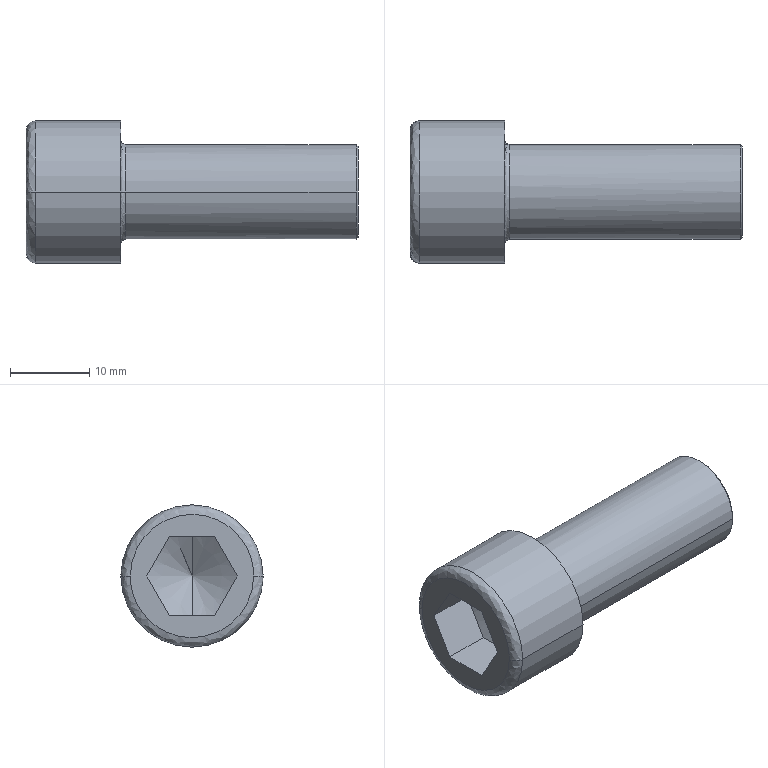Part | SolidWorks | features BaseBody 1 | 1 solid | 27 faces | box 42 x 18 x 18 mm | volume 5810 mm3 | plane 15 | spline 4 | cylinder 4 | cone 4 | commonest cylinder face diameters 12 x2 18 x2
STEP:
#1=CARTESIAN_POINT('',(0.6,6.,0.));
#2=VERTEX_POINT('',#1);
#3=CARTESIAN_POINT('',(0.6,-6.,0.));
#4=VERTEX_POINT('',#3);
#5=CARTESIAN_POINT('',(0.6,0.,0.));
#6=DIRECTION('',(1.,0.,0.));
#7=DIRECTION('',(0.,-1.,0.));
#8=AXIS2_PLACEMENT_3D('',#5,#6,#7);
#9=CIRCLE('',#8,6.);
#10=EDGE_CURVE('',#2,#4,#9,.T.);
#11=ORIENTED_EDGE('',*,*,#10,.F.);
#12=CARTESIAN_POINT('',(0.,6.6,0.));
#13=VERTEX_POINT('',#12);
#14=CARTESIAN_POINT('',(0.6,6.6,0.));
#15=DIRECTION('',(0.,0.,-1.));
#16=DIRECTION('',(0.,1.,0.));
#17=AXIS2_PLACEMENT_3D('',#14,#15,#16);
#18=CIRCLE('',#17,0.6);
#19=EDGE_CURVE('',#2,#13,#18,.T.);
#20=ORIENTED_EDGE('',*,*,#19,.T.);
#21=CARTESIAN_POINT('',(0.,-6.6,0.));
#22=VERTEX_POINT('',#21);
#23=CARTESIAN_POINT('',(0.,-6.6,0.));
#24=CARTESIAN_POINT('',(0.,-6.6,0.2019));
#25=CARTESIAN_POINT('',(0.,-6.586,0.5035));
#26=CARTESIAN_POINT('',(0.,-6.546,0.853));
#27=CARTESIAN_POINT('',(0.,-6.52,1.027));
#28=CARTESIAN_POINT('',(0.,-6.507,1.102));
#29=CARTESIAN_POINT('',(0.,-6.499,1.151));
#30=CARTESIAN_POINT('',(0.,-6.495,1.175));
#31=CARTESIAN_POINT('',(0.,-6.451,1.412));
#32=CARTESIAN_POINT('',(0.,-6.377,1.723));
#33=CARTESIAN_POINT('',(0.,-6.266,2.079));
#34=CARTESIAN_POINT('',(0.,-6.203,2.255));
#35=CARTESIAN_POINT('',(0.,-6.175,2.33));
#36=CARTESIAN_POINT('',(0.,-6.156,2.38));
#37=CARTESIAN_POINT('',(0.,-6.147,2.403));
#38=CARTESIAN_POINT('',(0.,-6.054,2.637));
#39=CARTESIAN_POINT('',(0.,-5.916,2.94));
#40=CARTESIAN_POINT('',(0.,-5.729,3.281));
#41=CARTESIAN_POINT('',(0.,-5.643,3.423));
#42=CARTESIAN_POINT('',(0.,-5.585,3.518));
#43=CARTESIAN_POINT('',(0.,-5.555,3.564));
#44=CARTESIAN_POINT('',(0.,-5.275,3.993));
#45=CARTESIAN_POINT('',(0.,-4.989,4.344));
#46=CARTESIAN_POINT('',(0.,-4.506,4.828));
#47=CARTESIAN_POINT('',(0.,-4.253,5.056));
#48=CARTESIAN_POINT('',(0.,-3.984,5.264));
#49=CARTESIAN_POINT('',(0.,-3.8,5.397));
#50=CARTESIAN_POINT('',(0.,-3.705,5.463));
#51=CARTESIAN_POINT('',(0.,-3.425,5.646));
#52=CARTESIAN_POINT('',(0.,-3.137,5.814));
#53=CARTESIAN_POINT('',(0.,-2.788,5.984));
#54=CARTESIAN_POINT('',(0.,-2.635,6.051));
#55=CARTESIAN_POINT('',(0.,-2.533,6.095));
#56=CARTESIAN_POINT('',(0.,-2.479,6.117));
#57=CARTESIAN_POINT('',(0.,-2.23,6.215));
#58=CARTESIAN_POINT('',(0.,-1.927,6.319));
#59=CARTESIAN_POINT('',(0.,-1.567,6.413));
#60=CARTESIAN_POINT('',(0.,-1.384,6.454));
#61=CARTESIAN_POINT('',(0.,-1.306,6.47));
#62=CARTESIAN_POINT('',(0.,-1.253,6.48));
#63=CARTESIAN_POINT('',(0.,-1.226,6.485));
#64=CARTESIAN_POINT('',(0.,-0.8037,6.563));
#65=CARTESIAN_POINT('',(0.,-0.404,6.6));
#66=CARTESIAN_POINT('',(0.,0.202,6.6));
#67=CARTESIAN_POINT('',(0.,0.5037,6.586));
#68=CARTESIAN_POINT('',(0.,0.8531,6.546));
#69=CARTESIAN_POINT('',(0.,1.027,6.52));
#70=CARTESIAN_POINT('',(0.,1.102,6.507));
#71=CARTESIAN_POINT('',(0.,1.151,6.499));
#72=CARTESIAN_POINT('',(0.,1.175,6.495));
#73=CARTESIAN_POINT('',(0.,1.412,6.451));
#74=CARTESIAN_POINT('',(0.,1.723,6.377));
#75=CARTESIAN_POINT('',(0.,2.079,6.266));
#76=CARTESIAN_POINT('',(0.,2.255,6.203));
#77=CARTESIAN_POINT('',(0.,2.33,6.175));
#78=CARTESIAN_POINT('',(0.,2.38,6.156));
#79=CARTESIAN_POINT('',(0.,2.403,6.147));
#80=CARTESIAN_POINT('',(0.,2.637,6.054));
#81=CARTESIAN_POINT('',(0.,2.94,5.916));
#82=CARTESIAN_POINT('',(0.,3.281,5.729));
#83=CARTESIAN_POINT('',(0.,3.423,5.643));
#84=CARTESIAN_POINT('',(0.,3.518,5.585));
#85=CARTESIAN_POINT('',(0.,3.564,5.555));
#86=CARTESIAN_POINT('',(0.,3.993,5.275));
#87=CARTESIAN_POINT('',(0.,4.344,4.989));
#88=CARTESIAN_POINT('',(0.,4.828,4.506));
#89=CARTESIAN_POINT('',(0.,5.056,4.253));
#90=CARTESIAN_POINT('',(0.,5.264,3.984));
#91=CARTESIAN_POINT('',(0.,5.397,3.8));
#92=CARTESIAN_POINT('',(0.,5.463,3.705));
#93=CARTESIAN_POINT('',(0.,5.646,3.425));
#94=CARTESIAN_POINT('',(0.,5.814,3.137));
#95=CARTESIAN_POINT('',(0.,5.984,2.788));
#96=CARTESIAN_POINT('',(0.,6.051,2.635));
#97=CARTESIAN_POINT('',(0.,6.095,2.533));
#98=CARTESIAN_POINT('',(0.,6.117,2.479));
#99=CARTESIAN_POINT('',(0.,6.215,2.23));
#100=CARTESIAN_POINT('',(0.,6.319,1.927));
#101=CARTESIAN_POINT('',(0.,6.413,1.567));
#102=CARTESIAN_POINT('',(0.,6.454,1.384));
#103=CARTESIAN_POINT('',(0.,6.47,1.306));
#104=CARTESIAN_POINT('',(0.,6.48,1.253));
#105=CARTESIAN_POINT('',(0.,6.485,1.226));
#106=CARTESIAN_POINT('',(0.,6.563,0.8038));
#107=CARTESIAN_POINT('',(0.,6.6,0.4035));
#108=CARTESIAN_POINT('',(0.,6.6,0.));
#109=B_SPLINE_CURVE_WITH_KNOTS('',3,(#23,#24,#25,#26,#27,#28,#29,#30,#31,#32,#33,#34,#35,#36,#37,#38,#39,#40,#41,#42,#43,#44,#45,#46,#47,#48,#49,#50,#51,#52,#53,#54,#55,#56,#57,#58,#59,#60,#61,#62,#63,#64,#65,#66,#67,#68,#69,#70,#71,#72,#73,#74,#75,#76,#77,#78,#79,#80,#81,#82,#83,#84,#85,#86,#87,#88,#89,#90,#91,#92,#93,#94,#95,#96,#97,#98,#99,#100,#101,#102,#103,#104,#105,#106,#107,#108),.UNSPECIFIED.,.F.,.F.,(4,1,1,1,2,2,1,1,1,2,2,1,1,2,2,2,1,2,2,1,1,2,2,1,1,1,2,2,2,1,1,1,2,2,1,1,1,2,2,1,1,2,2,2,1,2,2,1,1,2,2,1,1,1,2,2,4),(0.,0.03125,0.04688,0.05469,0.05859,0.0625,0.09375,0.1094,0.1172,0.1211,0.125,0.1563,0.1719,0.1797,0.1875,0.25,0.2813,0.2969,0.3125,0.3438,0.3594,0.3672,0.375,0.4063,0.4219,0.4297,0.4336,0.4375,0.5,0.5313,0.5469,0.5547,0.5586,0.5625,0.5938,0.6094,0.6172,0.6211,0.625,0.6563,0.6719,0.6797,0.6875,0.75,0.7813,0.7969,0.8125,0.8438,0.8594,0.8672,0.875,0.9063,0.9219,0.9297,0.9336,0.9375,1.),.UNSPECIFIED.);
#110=EDGE_CURVE('',#22,#13,#109,.T.);
#111=ORIENTED_EDGE('',*,*,#110,.F.);
#112=CARTESIAN_POINT('',(0.6,-6.6,0.));
#113=DIRECTION('',(0.,0.,1.));
#114=DIRECTION('',(0.,-1.,0.));
#115=AXIS2_PLACEMENT_3D('',#112,#113,#114);
#116=CIRCLE('',#115,0.6);
#117=EDGE_CURVE('',#4,#22,#116,.T.);
#118=ORIENTED_EDGE('',*,*,#117,.F.);
#119=EDGE_LOOP('',(#11,#20,#111,#118));
#120=FACE_OUTER_BOUND('',#119,.T.);
#121=CARTESIAN_POINT('',(0.6,-6.,0.));
#122=CARTESIAN_POINT('',(0.6,-6.,12.));
#123=CARTESIAN_POINT('',(0.6,6.,12.));
#124=CARTESIAN_POINT('',(0.6,6.,0.));
#125=CARTESIAN_POINT('',(0.2485,-6.,0.));
#126=CARTESIAN_POINT('',(0.2485,-6.,12.));
#127=CARTESIAN_POINT('',(0.2485,6.,12.));
#128=CARTESIAN_POINT('',(0.2485,6.,0.));
#129=CARTESIAN_POINT('',(0.,-6.249,0.));
#130=CARTESIAN_POINT('',(0.,-6.249,12.497));
#131=CARTESIAN_POINT('',(0.,6.249,12.497));
#132=CARTESIAN_POINT('',(0.,6.249,0.));
#133=CARTESIAN_POINT('',(0.,-6.6,0.));
#134=CARTESIAN_POINT('',(0.,-6.6,13.2));
#135=CARTESIAN_POINT('',(0.,6.6,13.2));
#136=CARTESIAN_POINT('',(0.,6.6,0.));
#137=(BOUNDED_SURFACE()B_SPLINE_SURFACE(3,3,((#121,#122,#123,#124),(#125,#126,#127,#128),(#129,#130,#131,#132),(#133,#134,#135,#136)),.UNSPECIFIED.,.F.,.F.,.T.)B_SPLINE_SURFACE_WITH_KNOTS((4,4),(4,4),(0.,1.),(0.,1.),.UNSPECIFIED.)GEOMETRIC_REPRESENTATION_ITEM()RATIONAL_B_SPLINE_SURFACE(((1.,0.3333,0.3333,1.),(0.8047,0.2682,0.2682,0.8047),(0.8047,0.2682,0.2682,0.8047),(1.,0.3333,0.3333,1.)))REPRESENTATION_ITEM('')SURFACE());
#138=ADVANCED_FACE('',(#120),#137,.F.);
#139=CARTESIAN_POINT('',(-10.8,-9.,0.));
#140=VERTEX_POINT('',#139);
#141=CARTESIAN_POINT('',(-10.8,9.,0.));
#142=VERTEX_POINT('',#141);
#143=CARTESIAN_POINT('',(-10.8,0.,0.));
#144=DIRECTION('',(1.,0.,0.));
#145=DIRECTION('',(0.,-1.,0.));
#146=AXIS2_PLACEMENT_3D('',#143,#144,#145);
#147=CIRCLE('',#146,9.);
#148=EDGE_CURVE('',#140,#142,#147,.T.);
#149=ORIENTED_EDGE('',*,*,#148,.F.);
#150=CARTESIAN_POINT('',(-12.,-7.8,0.));
#151=VERTEX_POINT('',#150);
#152=CARTESIAN_POINT('',(-10.8,-7.8,0.));
#153=DIRECTION('',(0.,0.,-1.));
#154=DIRECTION('',(0.,-1.,0.));
#155=AXIS2_PLACEMENT_3D('',#152,#153,#154);
#156=CIRCLE('',#155,1.2);
#157=EDGE_CURVE('',#140,#151,#156,.T.);
#158=ORIENTED_EDGE('',*,*,#157,.T.);
#159=CARTESIAN_POINT('',(-12.,7.8,0.));
#160=VERTEX_POINT('',#159);
#161=CARTESIAN_POINT('',(-12.,-7.8,0.));
#162=CARTESIAN_POINT('',(-12.,-7.8,-15.6));
#163=CARTESIAN_POINT('',(-12.,7.8,-15.6));
#164=CARTESIAN_POINT('',(-12.,7.8,0.));
#165=(BOUNDED_CURVE()B_SPLINE_CURVE(3,(#161,#162,#163,#164),.UNSPECIFIED.,.F.,.T.)B_SPLINE_CURVE_WITH_KNOTS((4,4),(0.,1.),.UNSPECIFIED.)CURVE()GEOMETRIC_REPRESENTATION_ITEM()RATIONAL_B_SPLINE_CURVE((1.,0.3333,0.3333,1.))REPRESENTATION_ITEM(''));
#166=EDGE_CURVE('',#151,#160,#165,.T.);
#167=ORIENTED_EDGE('',*,*,#166,.T.);
#168=CARTESIAN_POINT('',(-10.8,7.8,0.));
#169=DIRECTION('',(0.,0.,1.));
#170=DIRECTION('',(0.,1.,0.));
#171=AXIS2_PLACEMENT_3D('',#168,#169,#170);
#172=CIRCLE('',#171,1.2);
#173=EDGE_CURVE('',#142,#160,#172,.T.);
#174=ORIENTED_EDGE('',*,*,#173,.F.);
#175=EDGE_LOOP('',(#149,#158,#167,#174));
#176=FACE_OUTER_BOUND('',#175,.T.);
#177=CARTESIAN_POINT('',(-10.8,-9.,0.));
#178=CARTESIAN_POINT('',(-10.8,-9.,-18.));
#179=CARTESIAN_POINT('',(-10.8,9.,-18.));
#180=CARTESIAN_POINT('',(-10.8,9.,0.));
#181=CARTESIAN_POINT('',(-11.503,-9.,0.));
#182=CARTESIAN_POINT('',(-11.503,-9.,-18.));
#183=CARTESIAN_POINT('',(-11.503,9.,-18.));
#184=CARTESIAN_POINT('',(-11.503,9.,0.));
#185=CARTESIAN_POINT('',(-12.,-8.503,0.));
#186=CARTESIAN_POINT('',(-12.,-8.503,-17.006));
#187=CARTESIAN_POINT('',(-12.,8.503,-17.006));
#188=CARTESIAN_POINT('',(-12.,8.503,0.));
#189=CARTESIAN_POINT('',(-12.,-7.8,0.));
#190=CARTESIAN_POINT('',(-12.,-7.8,-15.6));
#191=CARTESIAN_POINT('',(-12.,7.8,-15.6));
#192=CARTESIAN_POINT('',(-12.,7.8,0.));
#193=(BOUNDED_SURFACE()B_SPLINE_SURFACE(3,3,((#177,#178,#179,#180),(#181,#182,#183,#184),(#185,#186,#187,#188),(#189,#190,#191,#192)),.UNSPECIFIED.,.F.,.F.,.F.)B_SPLINE_SURFACE_WITH_KNOTS((4,4),(4,4),(0.,1.),(0.,1.),.UNSPECIFIED.)GEOMETRIC_REPRESENTATION_ITEM()RATIONAL_B_SPLINE_SURFACE(((1.,0.3333,0.3333,1.),(0.8047,0.2682,0.2682,0.8047),(0.8047,0.2682,0.2682,0.8047),(1.,0.3333,0.3333,1.)))REPRESENTATION_ITEM('')SURFACE());
#194=ADVANCED_FACE('',(#176),#193,.T.);
#195=CARTESIAN_POINT('',(29.76,0.,6.));
#196=VERTEX_POINT('',#195);
#197=CARTESIAN_POINT('',(29.76,6.,0.));
#198=VERTEX_POINT('',#197);
#199=CARTESIAN_POINT('',(29.76,0.,0.));
#200=DIRECTION('',(-1.,0.,0.));
#201=DIRECTION('',(0.,-1.,0.));
#202=AXIS2_PLACEMENT_3D('',#199,#200,#201);
#203=CIRCLE('',#202,6.);
#204=EDGE_CURVE('',#196,#198,#203,.T.);
#205=ORIENTED_EDGE('',*,*,#204,.T.);
#206=CARTESIAN_POINT('',(30.,6.,0.));
#207=DIRECTION('',(-1.,0.,0.));
#208=VECTOR('',#207,1000.);
#209=LINE('',#206,#208);
#210=EDGE_CURVE('',#198,#2,#209,.T.);
#211=ORIENTED_EDGE('',*,*,#210,.T.);
#212=ORIENTED_EDGE('',*,*,#10,.T.);
#213=CARTESIAN_POINT('',(29.76,-6.,0.));
#214=VERTEX_POINT('',#213);
#215=CARTESIAN_POINT('',(30.,-6.,0.));
#216=DIRECTION('',(-1.,0.,0.));
#217=VECTOR('',#216,1000.);
#218=LINE('',#215,#217);
#219=EDGE_CURVE('',#214,#4,#218,.T.);
#220=ORIENTED_EDGE('',*,*,#219,.F.);
#221=CARTESIAN_POINT('',(29.76,0.,0.));
#222=DIRECTION('',(-1.,0.,0.));
#223=DIRECTION('',(0.,-1.,0.));
#224=AXIS2_PLACEMENT_3D('',#221,#222,#223);
#225=CIRCLE('',#224,6.);
#226=EDGE_CURVE('',#214,#196,#225,.T.);
#227=ORIENTED_EDGE('',*,*,#226,.T.);
#228=EDGE_LOOP('',(#205,#211,#212,#220,#227));
#229=FACE_OUTER_BOUND('',#228,.T.);
#230=CARTESIAN_POINT('',(30.,0.,0.));
#231=DIRECTION('',(-1.,0.,0.));
#232=DIRECTION('',(0.,-1.,0.));
#233=AXIS2_PLACEMENT_3D('',#230,#231,#232);
#234=CYLINDRICAL_SURFACE('',#233,6.);
#235=ADVANCED_FACE('',(#229),#234,.T.);
#236=CARTESIAN_POINT('',(30.,0.,5.76));
#237=VERTEX_POINT('',#236);
#238=CARTESIAN_POINT('',(30.,0.,-5.76));
#239=VERTEX_POINT('',#238);
#240=CARTESIAN_POINT('',(30.,0.,0.));
#241=DIRECTION('',(-1.,0.,0.));
#242=DIRECTION('',(0.,0.,1.));
#243=AXIS2_PLACEMENT_3D('',#240,#241,#242);
#244=CIRCLE('',#243,5.76);
#245=EDGE_CURVE('',#237,#239,#244,.T.);
#246=ORIENTED_EDGE('',*,*,#245,.T.);
#247=CARTESIAN_POINT('',(29.76,0.,-6.));
#248=VERTEX_POINT('',#247);
#249=CARTESIAN_POINT('',(29.76,0.,-6.));
#250=DIRECTION('',(-0.7071,0.,-0.7071));
#251=VECTOR('',#250,1000.);
#252=LINE('',#249,#251);
#253=EDGE_CURVE('',#239,#248,#252,.T.);
#254=ORIENTED_EDGE('',*,*,#253,.T.);
#255=CARTESIAN_POINT('',(29.76,0.,0.));
#256=DIRECTION('',(-1.,0.,0.));
#257=DIRECTION('',(0.,-1.,0.));
#258=AXIS2_PLACEMENT_3D('',#255,#256,#257);
#259=CIRCLE('',#258,6.);
#260=EDGE_CURVE('',#198,#248,#259,.T.);
#261=ORIENTED_EDGE('',*,*,#260,.F.);
#262=ORIENTED_EDGE('',*,*,#204,.F.);
#263=CARTESIAN_POINT('',(29.76,0.,6.));
#264=DIRECTION('',(-0.7071,0.,0.7071));
#265=VECTOR('',#264,1000.);
#266=LINE('',#263,#265);
#267=EDGE_CURVE('',#237,#196,#266,.T.);
#268=ORIENTED_EDGE('',*,*,#267,.F.);
#269=EDGE_LOOP('',(#246,#254,#261,#262,#268));
#270=FACE_OUTER_BOUND('',#269,.T.);
#271=CARTESIAN_POINT('',(29.76,0.,0.));
#272=DIRECTION('',(-1.,0.,0.));
#273=DIRECTION('',(0.,0.,1.));
#274=AXIS2_PLACEMENT_3D('',#271,#272,#273);
#275=CONICAL_SURFACE('',#274,6.,0.7854);
#276=ADVANCED_FACE('',(#270),#275,.T.);
#277=CARTESIAN_POINT('',(0.,-9.,0.));
#278=VERTEX_POINT('',#277);
#279=CARTESIAN_POINT('',(0.,9.,0.));
#280=VERTEX_POINT('',#279);
#281=CARTESIAN_POINT('',(0.,0.,0.));
#282=DIRECTION('',(-1.,0.,0.));
#283=DIRECTION('',(0.,-1.,0.));
#284=AXIS2_PLACEMENT_3D('',#281,#282,#283);
#285=CIRCLE('',#284,9.);
#286=EDGE_CURVE('',#278,#280,#285,.T.);
#287=ORIENTED_EDGE('',*,*,#286,.T.);
#288=CARTESIAN_POINT('',(-2.701,9.,0.));
#289=DIRECTION('',(-1.,0.,0.));
#290=VECTOR('',#289,1000.);
#291=LINE('',#288,#290);
#292=EDGE_CURVE('',#280,#142,#291,.T.);
#293=ORIENTED_EDGE('',*,*,#292,.T.);
#294=CARTESIAN_POINT('',(-10.8,0.,0.));
#295=DIRECTION('',(1.,0.,0.));
#296=DIRECTION('',(0.,-1.,0.));
#297=AXIS2_PLACEMENT_3D('',#294,#295,#296);
#298=CIRCLE('',#297,9.);
#299=EDGE_CURVE('',#142,#140,#298,.T.);
#300=ORIENTED_EDGE('',*,*,#299,.T.);
#301=CARTESIAN_POINT('',(-2.701,-9.,0.));
#302=DIRECTION('',(-1.,0.,0.));
#303=VECTOR('',#302,1000.);
#304=LINE('',#301,#303);
#305=EDGE_CURVE('',#278,#140,#304,.T.);
#306=ORIENTED_EDGE('',*,*,#305,.F.);
#307=EDGE_LOOP('',(#287,#293,#300,#306));
#308=FACE_OUTER_BOUND('',#307,.T.);
#309=CARTESIAN_POINT('',(-2.701,0.,0.));
#310=DIRECTION('',(-1.,0.,0.));
#311=DIRECTION('',(0.,-1.,0.));
#312=AXIS2_PLACEMENT_3D('',#309,#310,#311);
#313=CYLINDRICAL_SURFACE('',#312,9.);
#314=ADVANCED_FACE('',(#308),#313,.T.);
#315=CARTESIAN_POINT('',(-2.701,0.,0.));
#316=VERTEX_POINT('',#315);
#317=CARTESIAN_POINT('',(-6.,0.,5.715));
#318=VERTEX_POINT('',#317);
#319=CARTESIAN_POINT('',(-6.,0.,5.715));
#320=DIRECTION('',(-0.5,0.,0.866));
#321=VECTOR('',#320,1000.);
#322=LINE('',#319,#321);
#323=EDGE_CURVE('',#316,#318,#322,.T.);
#324=ORIENTED_EDGE('',*,*,#323,.F.);
#325=CARTESIAN_POINT('',(-6.,0.,-5.714));
#326=VERTEX_POINT('',#325);
#327=CARTESIAN_POINT('',(-6.,0.,-5.715));
#328=DIRECTION('',(-0.5,0.,-0.866));
#329=VECTOR('',#328,1000.);
#330=LINE('',#327,#329);
#331=EDGE_CURVE('',#316,#326,#330,.T.);
#332=ORIENTED_EDGE('',*,*,#331,.T.);
#333=CARTESIAN_POINT('',(-6.,-2.857,-4.949));
#334=VERTEX_POINT('',#333);
#335=CARTESIAN_POINT('',(-6.,0.,0.));
#336=DIRECTION('',(-1.,0.,0.));
#337=DIRECTION('',(0.,0.,1.));
#338=AXIS2_PLACEMENT_3D('',#335,#336,#337);
#339=CIRCLE('',#338,5.715);
#340=EDGE_CURVE('',#326,#334,#339,.T.);
#341=ORIENTED_EDGE('',*,*,#340,.T.);
#342=CARTESIAN_POINT('',(-6.,-5.715,0.));
#343=VERTEX_POINT('',#342);
#344=CARTESIAN_POINT('',(-6.,0.,0.));
#345=DIRECTION('',(-1.,0.,0.));
#346=DIRECTION('',(0.,0.,1.));
#347=AXIS2_PLACEMENT_3D('',#344,#345,#346);
#348=CIRCLE('',#347,5.715);
#349=EDGE_CURVE('',#334,#343,#348,.T.);
#350=ORIENTED_EDGE('',*,*,#349,.T.);
#351=CARTESIAN_POINT('',(-6.,-2.857,4.949));
#352=VERTEX_POINT('',#351);
#353=CARTESIAN_POINT('',(-6.,0.,0.));
#354=DIRECTION('',(-1.,0.,0.));
#355=DIRECTION('',(0.,0.,1.));
#356=AXIS2_PLACEMENT_3D('',#353,#354,#355);
#357=CIRCLE('',#356,5.715);
#358=EDGE_CURVE('',#343,#352,#357,.T.);
#359=ORIENTED_EDGE('',*,*,#358,.T.);
#360=CARTESIAN_POINT('',(-6.,0.,0.));
#361=DIRECTION('',(-1.,0.,0.));
#362=DIRECTION('',(0.,0.,1.));
#363=AXIS2_PLACEMENT_3D('',#360,#361,#362);
#364=CIRCLE('',#363,5.715);
#365=EDGE_CURVE('',#352,#318,#364,.T.);
#366=ORIENTED_EDGE('',*,*,#365,.T.);
#367=EDGE_LOOP('',(#324,#332,#341,#350,#359,#366));
#368=FACE_OUTER_BOUND('',#367,.T.);
#369=CARTESIAN_POINT('',(-6.,0.,0.));
#370=DIRECTION('',(-1.,0.,0.));
#371=DIRECTION('',(0.,0.,1.));
#372=AXIS2_PLACEMENT_3D('',#369,#370,#371);
#373=CONICAL_SURFACE('',#372,5.715,1.047);
#374=ADVANCED_FACE('',(#368),#373,.F.);
#375=ORIENTED_EDGE('',*,*,#210,.F.);
#376=ORIENTED_EDGE('',*,*,#260,.T.);
#377=CARTESIAN_POINT('',(29.76,0.,0.));
#378=DIRECTION('',(-1.,0.,0.));
#379=DIRECTION('',(0.,-1.,0.));
#380=AXIS2_PLACEMENT_3D('',#377,#378,#379);
#381=CIRCLE('',#380,6.);
#382=EDGE_CURVE('',#248,#214,#381,.T.);
#383=ORIENTED_EDGE('',*,*,#382,.T.);
#384=ORIENTED_EDGE('',*,*,#219,.T.);
#385=CARTESIAN_POINT('',(0.6,0.,0.));
#386=DIRECTION('',(1.,0.,0.));
#387=DIRECTION('',(0.,-1.,0.));
#388=AXIS2_PLACEMENT_3D('',#385,#386,#387);
#389=CIRCLE('',#388,6.);
#390=EDGE_CURVE('',#4,#2,#389,.T.);
#391=ORIENTED_EDGE('',*,*,#390,.T.);
#392=EDGE_LOOP('',(#375,#376,#383,#384,#391));
#393=FACE_OUTER_BOUND('',#392,.T.);
#394=CARTESIAN_POINT('',(30.,0.,0.));
#395=DIRECTION('',(-1.,0.,0.));
#396=DIRECTION('',(0.,-1.,0.));
#397=AXIS2_PLACEMENT_3D('',#394,#395,#396);
#398=CYLINDRICAL_SURFACE('',#397,6.);
#399=ADVANCED_FACE('',(#393),#398,.T.);
#400=ORIENTED_EDGE('',*,*,#19,.F.);
#401=ORIENTED_EDGE('',*,*,#390,.F.);
#402=ORIENTED_EDGE('',*,*,#117,.T.);
#403=CARTESIAN_POINT('',(0.,6.6,0.));
#404=CARTESIAN_POINT('',(0.,6.6,-0.2019));
#405=CARTESIAN_POINT('',(0.,6.586,-0.5035));
#406=CARTESIAN_POINT('',(0.,6.546,-0.853));
#407=CARTESIAN_POINT('',(0.,6.52,-1.027));
#408=CARTESIAN_POINT('',(0.,6.507,-1.102));
#409=CARTESIAN_POINT('',(0.,6.499,-1.151));
#410=CARTESIAN_POINT('',(0.,6.495,-1.175));
#411=CARTESIAN_POINT('',(0.,6.451,-1.412));
#412=CARTESIAN_POINT('',(0.,6.377,-1.723));
#413=CARTESIAN_POINT('',(0.,6.266,-2.079));
#414=CARTESIAN_POINT('',(0.,6.203,-2.255));
#415=CARTESIAN_POINT('',(0.,6.175,-2.33));
#416=CARTESIAN_POINT('',(0.,6.156,-2.38));
#417=CARTESIAN_POINT('',(0.,6.147,-2.403));
#418=CARTESIAN_POINT('',(0.,6.054,-2.637));
#419=CARTESIAN_POINT('',(0.,5.916,-2.94));
#420=CARTESIAN_POINT('',(0.,5.729,-3.281));
#421=CARTESIAN_POINT('',(0.,5.643,-3.423));
#422=CARTESIAN_POINT('',(0.,5.585,-3.518));
#423=CARTESIAN_POINT('',(0.,5.555,-3.564));
#424=CARTESIAN_POINT('',(0.,5.275,-3.993));
#425=CARTESIAN_POINT('',(0.,4.989,-4.344));
#426=CARTESIAN_POINT('',(0.,4.506,-4.828));
#427=CARTESIAN_POINT('',(0.,4.253,-5.056));
#428=CARTESIAN_POINT('',(0.,3.984,-5.264));
#429=CARTESIAN_POINT('',(0.,3.8,-5.397));
#430=CARTESIAN_POINT('',(0.,3.705,-5.463));
#431=CARTESIAN_POINT('',(0.,3.425,-5.646));
#432=CARTESIAN_POINT('',(0.,3.137,-5.814));
#433=CARTESIAN_POINT('',(0.,2.788,-5.984));
#434=CARTESIAN_POINT('',(0.,2.635,-6.051));
#435=CARTESIAN_POINT('',(0.,2.533,-6.095));
#436=CARTESIAN_POINT('',(0.,2.479,-6.117));
#437=CARTESIAN_POINT('',(0.,2.23,-6.215));
#438=CARTESIAN_POINT('',(0.,1.927,-6.319));
#439=CARTESIAN_POINT('',(0.,1.567,-6.413));
#440=CARTESIAN_POINT('',(0.,1.384,-6.454));
#441=CARTESIAN_POINT('',(0.,1.306,-6.47));
#442=CARTESIAN_POINT('',(0.,1.253,-6.48));
#443=CARTESIAN_POINT('',(0.,1.226,-6.485));
#444=CARTESIAN_POINT('',(0.,0.8037,-6.563));
#445=CARTESIAN_POINT('',(0.,0.404,-6.6));
#446=CARTESIAN_POINT('',(0.,-0.202,-6.6));
#447=CARTESIAN_POINT('',(0.,-0.5037,-6.586));
#448=CARTESIAN_POINT('',(0.,-0.8531,-6.546));
#449=CARTESIAN_POINT('',(0.,-1.027,-6.52));
#450=CARTESIAN_POINT('',(0.,-1.102,-6.507));
#451=CARTESIAN_POINT('',(0.,-1.151,-6.499));
#452=CARTESIAN_POINT('',(0.,-1.175,-6.495));
#453=CARTESIAN_POINT('',(0.,-1.412,-6.451));
#454=CARTESIAN_POINT('',(0.,-1.723,-6.377));
#455=CARTESIAN_POINT('',(0.,-2.079,-6.266));
#456=CARTESIAN_POINT('',(0.,-2.255,-6.203));
#457=CARTESIAN_POINT('',(0.,-2.33,-6.175));
#458=CARTESIAN_POINT('',(0.,-2.38,-6.156));
#459=CARTESIAN_POINT('',(0.,-2.403,-6.147));
#460=CARTESIAN_POINT('',(0.,-2.637,-6.054));
#461=CARTESIAN_POINT('',(0.,-2.94,-5.916));
#462=CARTESIAN_POINT('',(0.,-3.281,-5.729));
#463=CARTESIAN_POINT('',(0.,-3.423,-5.643));
#464=CARTESIAN_POINT('',(0.,-3.518,-5.585));
#465=CARTESIAN_POINT('',(0.,-3.564,-5.555));
#466=CARTESIAN_POINT('',(0.,-3.993,-5.275));
#467=CARTESIAN_POINT('',(0.,-4.344,-4.989));
#468=CARTESIAN_POINT('',(0.,-4.828,-4.506));
#469=CARTESIAN_POINT('',(0.,-5.056,-4.253));
#470=CARTESIAN_POINT('',(0.,-5.264,-3.984));
#471=CARTESIAN_POINT('',(0.,-5.397,-3.8));
#472=CARTESIAN_POINT('',(0.,-5.463,-3.705));
#473=CARTESIAN_POINT('',(0.,-5.646,-3.425));
#474=CARTESIAN_POINT('',(0.,-5.814,-3.137));
#475=CARTESIAN_POINT('',(0.,-5.984,-2.788));
#476=CARTESIAN_POINT('',(0.,-6.051,-2.635));
#477=CARTESIAN_POINT('',(0.,-6.095,-2.533));
#478=CARTESIAN_POINT('',(0.,-6.117,-2.479));
#479=CARTESIAN_POINT('',(0.,-6.215,-2.23));
#480=CARTESIAN_POINT('',(0.,-6.319,-1.927));
#481=CARTESIAN_POINT('',(0.,-6.413,-1.567));
#482=CARTESIAN_POINT('',(0.,-6.454,-1.384));
#483=CARTESIAN_POINT('',(0.,-6.47,-1.306));
#484=CARTESIAN_POINT('',(0.,-6.48,-1.253));
#485=CARTESIAN_POINT('',(0.,-6.485,-1.226));
#486=CARTESIAN_POINT('',(0.,-6.563,-0.8038));
#487=CARTESIAN_POINT('',(0.,-6.6,-0.4035));
#488=CARTESIAN_POINT('',(0.,-6.6,0.));
#489=B_SPLINE_CURVE_WITH_KNOTS('',3,(#403,#404,#405,#406,#407,#408,#409,#410,#411,#412,#413,#414,#415,#416,#417,#418,#419,#420,#421,#422,#423,#424,#425,#426,#427,#428,#429,#430,#431,#432,#433,#434,#435,#436,#437,#438,#439,#440,#441,#442,#443,#444,#445,#446,#447,#448,#449,#450,#451,#452,#453,#454,#455,#456,#457,#458,#459,#460,#461,#462,#463,#464,#465,#466,#467,#468,#469,#470,#471,#472,#473,#474,#475,#476,#477,#478,#479,#480,#481,#482,#483,#484,#485,#486,#487,#488),.UNSPECIFIED.,.F.,.F.,(4,1,1,1,2,2,1,1,1,2,2,1,1,2,2,2,1,2,2,1,1,2,2,1,1,1,2,2,2,1,1,1,2,2,1,1,1,2,2,1,1,2,2,2,1,2,2,1,1,2,2,1,1,1,2,2,4),(0.,0.03125,0.04688,0.05469,0.05859,0.0625,0.09375,0.1094,0.1172,0.1211,0.125,0.1563,0.1719,0.1797,0.1875,0.25,0.2813,0.2969,0.3125,0.3437,0.3594,0.3672,0.375,0.4062,0.4219,0.4297,0.4336,0.4375,0.5,0.5312,0.5469,0.5547,0.5586,0.5625,0.5937,0.6094,0.6172,0.6211,0.625,0.6562,0.6719,0.6797,0.6875,0.75,0.7812,0.7969,0.8125,0.8437,0.8594,0.8672,0.875,0.9062,0.9219,0.9297,0.9336,0.9375,1.),.UNSPECIFIED.);
#490=EDGE_CURVE('',#13,#22,#489,.T.);
#491=ORIENTED_EDGE('',*,*,#490,.F.);
#492=EDGE_LOOP('',(#400,#401,#402,#491));
#493=FACE_OUTER_BOUND('',#492,.T.);
#494=CARTESIAN_POINT('',(0.6,6.,0.));
#495=CARTESIAN_POINT('',(0.6,6.,-12.));
#496=CARTESIAN_POINT('',(0.6,-6.,-12.));
#497=CARTESIAN_POINT('',(0.6,-6.,0.));
#498=CARTESIAN_POINT('',(0.2485,6.,0.));
#499=CARTESIAN_POINT('',(0.2485,6.,-12.));
#500=CARTESIAN_POINT('',(0.2485,-6.,-12.));
#501=CARTESIAN_POINT('',(0.2485,-6.,0.));
#502=CARTESIAN_POINT('',(0.,6.249,0.));
#503=CARTESIAN_POINT('',(0.,6.249,-12.497));
#504=CARTESIAN_POINT('',(0.,-6.249,-12.497));
#505=CARTESIAN_POINT('',(0.,-6.249,0.));
#506=CARTESIAN_POINT('',(0.,6.6,0.));
#507=CARTESIAN_POINT('',(0.,6.6,-13.2));
#508=CARTESIAN_POINT('',(0.,-6.6,-13.2));
#509=CARTESIAN_POINT('',(0.,-6.6,0.));
#510=(BOUNDED_SURFACE()B_SPLINE_SURFACE(3,3,((#494,#495,#496,#497),(#498,#499,#500,#501),(#502,#503,#504,#505),(#506,#507,#508,#509)),.UNSPECIFIED.,.F.,.F.,.F.)B_SPLINE_SURFACE_WITH_KNOTS((4,4),(4,4),(0.,1.),(0.,1.),.UNSPECIFIED.)GEOMETRIC_REPRESENTATION_ITEM()RATIONAL_B_SPLINE_SURFACE(((1.,0.3333,0.3333,1.),(0.8047,0.2682,0.2682,0.8047),(0.8047,0.2682,0.2682,0.8047),(1.,0.3333,0.3333,1.)))REPRESENTATION_ITEM('')SURFACE());
#511=ADVANCED_FACE('',(#493),#510,.F.);
#512=ORIENTED_EDGE('',*,*,#253,.F.);
#513=CARTESIAN_POINT('',(30.,0.,0.));
#514=DIRECTION('',(-1.,0.,0.));
#515=DIRECTION('',(0.,0.,1.));
#516=AXIS2_PLACEMENT_3D('',#513,#514,#515);
#517=CIRCLE('',#516,5.76);
#518=EDGE_CURVE('',#239,#237,#517,.T.);
#519=ORIENTED_EDGE('',*,*,#518,.T.);
#520=ORIENTED_EDGE('',*,*,#267,.T.);
#521=ORIENTED_EDGE('',*,*,#226,.F.);
#522=ORIENTED_EDGE('',*,*,#382,.F.);
#523=EDGE_LOOP('',(#512,#519,#520,#521,#522));
#524=FACE_OUTER_BOUND('',#523,.T.);
#525=CARTESIAN_POINT('',(29.76,0.,0.));
#526=DIRECTION('',(-1.,0.,0.));
#527=DIRECTION('',(0.,0.,1.));
#528=AXIS2_PLACEMENT_3D('',#525,#526,#527);
#529=CONICAL_SURFACE('',#528,6.,0.7854);
#530=ADVANCED_FACE('',(#524),#529,.T.);
#531=ORIENTED_EDGE('',*,*,#286,.F.);
#532=CARTESIAN_POINT('',(0.,0.,0.));
#533=DIRECTION('',(-1.,0.,0.));
#534=DIRECTION('',(0.,-1.,0.));
#535=AXIS2_PLACEMENT_3D('',#532,#533,#534);
#536=CIRCLE('',#535,9.);
#537=EDGE_CURVE('',#280,#278,#536,.T.);
#538=ORIENTED_EDGE('',*,*,#537,.F.);
#539=EDGE_LOOP('',(#531,#538));
#540=FACE_OUTER_BOUND('',#539,.T.);
#541=ORIENTED_EDGE('',*,*,#490,.T.);
#542=ORIENTED_EDGE('',*,*,#110,.T.);
#543=EDGE_LOOP('',(#541,#542));
#544=FACE_BOUND('',#543,.T.);
#545=CARTESIAN_POINT('',(0.,9.,0.));
#546=DIRECTION('',(-1.,0.,0.));
#547=DIRECTION('',(0.,-1.,0.));
#548=AXIS2_PLACEMENT_3D('',#545,#546,#547);
#549=PLANE('',#548);
#550=ADVANCED_FACE('',(#540,#544),#549,.F.);
#551=ORIENTED_EDGE('',*,*,#245,.F.);
#552=ORIENTED_EDGE('',*,*,#518,.F.);
#553=EDGE_LOOP('',(#551,#552));
#554=FACE_OUTER_BOUND('',#553,.T.);
#555=CARTESIAN_POINT('',(30.,0.,0.));
#556=DIRECTION('',(1.,0.,0.));
#557=DIRECTION('',(0.,1.,0.));
#558=AXIS2_PLACEMENT_3D('',#555,#556,#557);
#559=PLANE('',#558);
#560=ADVANCED_FACE('',(#554),#559,.T.);
#561=ORIENTED_EDGE('',*,*,#292,.F.);
#562=ORIENTED_EDGE('',*,*,#537,.T.);
#563=ORIENTED_EDGE('',*,*,#305,.T.);
#564=ORIENTED_EDGE('',*,*,#148,.T.);
#565=EDGE_LOOP('',(#561,#562,#563,#564));
#566=FACE_OUTER_BOUND('',#565,.T.);
#567=CARTESIAN_POINT('',(-2.701,0.,0.));
#568=DIRECTION('',(-1.,0.,0.));
#569=DIRECTION('',(0.,-1.,0.));
#570=AXIS2_PLACEMENT_3D('',#567,#568,#569);
#571=CYLINDRICAL_SURFACE('',#570,9.);
#572=ADVANCED_FACE('',(#566),#571,.T.);
#573=ORIENTED_EDGE('',*,*,#157,.F.);
#574=ORIENTED_EDGE('',*,*,#299,.F.);
#575=ORIENTED_EDGE('',*,*,#173,.T.);
#576=CARTESIAN_POINT('',(-12.,7.8,0.));
#577=CARTESIAN_POINT('',(-12.,7.8,15.6));
#578=CARTESIAN_POINT('',(-12.,-7.8,15.6));
#579=CARTESIAN_POINT('',(-12.,-7.8,0.));
#580=(BOUNDED_CURVE()B_SPLINE_CURVE(3,(#576,#577,#578,#579),.UNSPECIFIED.,.F.,.F.)B_SPLINE_CURVE_WITH_KNOTS((4,4),(0.,1.),.UNSPECIFIED.)CURVE()GEOMETRIC_REPRESENTATION_ITEM()RATIONAL_B_SPLINE_CURVE((1.,0.3333,0.3333,1.))REPRESENTATION_ITEM(''));
#581=EDGE_CURVE('',#160,#151,#580,.T.);
#582=ORIENTED_EDGE('',*,*,#581,.T.);
#583=EDGE_LOOP('',(#573,#574,#575,#582));
#584=FACE_OUTER_BOUND('',#583,.T.);
#585=CARTESIAN_POINT('',(-10.8,9.,0.));
#586=CARTESIAN_POINT('',(-10.8,9.,18.));
#587=CARTESIAN_POINT('',(-10.8,-9.,18.));
#588=CARTESIAN_POINT('',(-10.8,-9.,0.));
#589=CARTESIAN_POINT('',(-11.503,9.,0.));
#590=CARTESIAN_POINT('',(-11.503,9.,18.));
#591=CARTESIAN_POINT('',(-11.503,-9.,18.));
#592=CARTESIAN_POINT('',(-11.503,-9.,0.));
#593=CARTESIAN_POINT('',(-12.,8.503,0.));
#594=CARTESIAN_POINT('',(-12.,8.503,17.006));
#595=CARTESIAN_POINT('',(-12.,-8.503,17.006));
#596=CARTESIAN_POINT('',(-12.,-8.503,0.));
#597=CARTESIAN_POINT('',(-12.,7.8,0.));
#598=CARTESIAN_POINT('',(-12.,7.8,15.6));
#599=CARTESIAN_POINT('',(-12.,-7.8,15.6));
#600=CARTESIAN_POINT('',(-12.,-7.8,0.));
#601=(BOUNDED_SURFACE()B_SPLINE_SURFACE(3,3,((#585,#586,#587,#588),(#589,#590,#591,#592),(#593,#594,#595,#596),(#597,#598,#599,#600)),.UNSPECIFIED.,.F.,.F.,.F.)B_SPLINE_SURFACE_WITH_KNOTS((4,4),(4,4),(0.,1.),(0.,1.),.UNSPECIFIED.)GEOMETRIC_REPRESENTATION_ITEM()RATIONAL_B_SPLINE_SURFACE(((1.,0.3333,0.3333,1.),(0.8047,0.2682,0.2682,0.8047),(0.8047,0.2682,0.2682,0.8047),(1.,0.3333,0.3333,1.)))REPRESENTATION_ITEM('')SURFACE());
#602=ADVANCED_FACE('',(#584),#601,.T.);
#603=CARTESIAN_POINT('',(-12.,2.857,-4.949));
#604=VERTEX_POINT('',#603);
#605=CARTESIAN_POINT('',(-12.,-2.857,-4.949));
#606=VERTEX_POINT('',#605);
#607=CARTESIAN_POINT('',(-12.,5.715,-4.949));
#608=DIRECTION('',(0.,-1.,0.));
#609=VECTOR('',#608,1000.);
#610=LINE('',#607,#609);
#611=EDGE_CURVE('',#604,#606,#610,.T.);
#612=ORIENTED_EDGE('',*,*,#611,.F.);
#613=CARTESIAN_POINT('',(-12.,5.715,0.));
#614=VERTEX_POINT('',#613);
#615=CARTESIAN_POINT('',(-12.,5.715,0.));
#616=DIRECTION('',(0.,-0.5,-0.866));
#617=VECTOR('',#616,1000.);
#618=LINE('',#615,#617);
#619=EDGE_CURVE('',#614,#604,#618,.T.);
#620=ORIENTED_EDGE('',*,*,#619,.F.);
#621=CARTESIAN_POINT('',(-12.,2.857,4.949));
#622=VERTEX_POINT('',#621);
#623=CARTESIAN_POINT('',(-12.,2.857,4.949));
#624=DIRECTION('',(0.,0.5,-0.866));
#625=VECTOR('',#624,1000.);
#626=LINE('',#623,#625);
#627=EDGE_CURVE('',#622,#614,#626,.T.);
#628=ORIENTED_EDGE('',*,*,#627,.F.);
#629=CARTESIAN_POINT('',(-12.,-2.857,4.949));
#630=VERTEX_POINT('',#629);
#631=CARTESIAN_POINT('',(-12.,5.715,4.949));
#632=DIRECTION('',(0.,1.,0.));
#633=VECTOR('',#632,1000.);
#634=LINE('',#631,#633);
#635=EDGE_CURVE('',#630,#622,#634,.T.);
#636=ORIENTED_EDGE('',*,*,#635,.F.);
#637=CARTESIAN_POINT('',(-12.,-5.715,0.));
#638=VERTEX_POINT('',#637);
#639=CARTESIAN_POINT('',(-12.,-5.715,0.));
#640=DIRECTION('',(0.,0.5,0.866));
#641=VECTOR('',#640,1000.);
#642=LINE('',#639,#641);
#643=EDGE_CURVE('',#638,#630,#642,.T.);
#644=ORIENTED_EDGE('',*,*,#643,.F.);
#645=CARTESIAN_POINT('',(-12.,-2.857,-4.949));
#646=DIRECTION('',(0.,-0.5,0.866));
#647=VECTOR('',#646,1000.);
#648=LINE('',#645,#647);
#649=EDGE_CURVE('',#606,#638,#648,.T.);
#650=ORIENTED_EDGE('',*,*,#649,.F.);
#651=EDGE_LOOP('',(#612,#620,#628,#636,#644,#650));
#652=FACE_BOUND('',#651,.T.);
#653=ORIENTED_EDGE('',*,*,#581,.F.);
#654=ORIENTED_EDGE('',*,*,#166,.F.);
#655=EDGE_LOOP('',(#653,#654));
#656=FACE_OUTER_BOUND('',#655,.T.);
#657=CARTESIAN_POINT('',(-12.,5.715,0.));
#658=DIRECTION('',(1.,0.,0.));
#659=DIRECTION('',(0.,1.,0.));
#660=AXIS2_PLACEMENT_3D('',#657,#658,#659);
#661=PLANE('',#660);
#662=ADVANCED_FACE('',(#652,#656),#661,.F.);
#663=CARTESIAN_POINT('',(-6.,-2.857,-4.949));
#664=DIRECTION('',(0.,-0.5,0.866));
#665=VECTOR('',#664,1000.);
#666=LINE('',#663,#665);
#667=EDGE_CURVE('',#334,#343,#666,.T.);
#668=ORIENTED_EDGE('',*,*,#667,.F.);
#669=CARTESIAN_POINT('',(-6.,-2.857,-4.949));
#670=DIRECTION('',(1.,0.,0.));
#671=VECTOR('',#670,1000.);
#672=LINE('',#669,#671);
#673=EDGE_CURVE('',#606,#334,#672,.T.);
#674=ORIENTED_EDGE('',*,*,#673,.F.);
#675=ORIENTED_EDGE('',*,*,#649,.T.);
#676=CARTESIAN_POINT('',(-6.,-5.715,0.));
#677=DIRECTION('',(-1.,0.,0.));
#678=VECTOR('',#677,1000.);
#679=LINE('',#676,#678);
#680=EDGE_CURVE('',#343,#638,#679,.T.);
#681=ORIENTED_EDGE('',*,*,#680,.F.);
#682=EDGE_LOOP('',(#668,#674,#675,#681));
#683=FACE_OUTER_BOUND('',#682,.T.);
#684=CARTESIAN_POINT('',(-6.,-2.857,-4.949));
#685=DIRECTION('',(0.,-0.866,-0.5));
#686=DIRECTION('',(0.,0.5,-0.866));
#687=AXIS2_PLACEMENT_3D('',#684,#685,#686);
#688=PLANE('',#687);
#689=ADVANCED_FACE('',(#683),#688,.F.);
#690=CARTESIAN_POINT('',(-6.,2.857,-4.949));
#691=VERTEX_POINT('',#690);
#692=CARTESIAN_POINT('',(-6.,2.857,-4.949));
#693=DIRECTION('',(0.,-1.,0.));
#694=VECTOR('',#693,1000.);
#695=LINE('',#692,#694);
#696=EDGE_CURVE('',#691,#334,#695,.T.);
#697=ORIENTED_EDGE('',*,*,#696,.F.);
#698=CARTESIAN_POINT('',(-6.,2.857,-4.949));
#699=DIRECTION('',(1.,0.,0.));
#700=VECTOR('',#699,1000.);
#701=LINE('',#698,#700);
#702=EDGE_CURVE('',#604,#691,#701,.T.);
#703=ORIENTED_EDGE('',*,*,#702,.F.);
#704=ORIENTED_EDGE('',*,*,#611,.T.);
#705=ORIENTED_EDGE('',*,*,#673,.T.);
#706=EDGE_LOOP('',(#697,#703,#704,#705));
#707=FACE_OUTER_BOUND('',#706,.T.);
#708=CARTESIAN_POINT('',(-6.,2.857,-4.949));
#709=DIRECTION('',(0.,0.,-1.));
#710=DIRECTION('',(0.,1.,0.));
#711=AXIS2_PLACEMENT_3D('',#708,#709,#710);
#712=PLANE('',#711);
#713=ADVANCED_FACE('',(#707),#712,.F.);
#714=CARTESIAN_POINT('',(-6.,5.715,0.));
#715=VERTEX_POINT('',#714);
#716=CARTESIAN_POINT('',(-6.,5.715,0.));
#717=DIRECTION('',(0.,-0.5,-0.866));
#718=VECTOR('',#717,1000.);
#719=LINE('',#716,#718);
#720=EDGE_CURVE('',#715,#691,#719,.T.);
#721=ORIENTED_EDGE('',*,*,#720,.F.);
#722=CARTESIAN_POINT('',(-6.,5.715,0.));
#723=DIRECTION('',(1.,0.,0.));
#724=VECTOR('',#723,1000.);
#725=LINE('',#722,#724);
#726=EDGE_CURVE('',#614,#715,#725,.T.);
#727=ORIENTED_EDGE('',*,*,#726,.F.);
#728=ORIENTED_EDGE('',*,*,#619,.T.);
#729=ORIENTED_EDGE('',*,*,#702,.T.);
#730=EDGE_LOOP('',(#721,#727,#728,#729));
#731=FACE_OUTER_BOUND('',#730,.T.);
#732=CARTESIAN_POINT('',(-6.,5.715,0.));
#733=DIRECTION('',(0.,0.866,-0.5));
#734=DIRECTION('',(0.,0.5,0.866));
#735=AXIS2_PLACEMENT_3D('',#732,#733,#734);
#736=PLANE('',#735);
#737=ADVANCED_FACE('',(#731),#736,.F.);
#738=CARTESIAN_POINT('',(-6.,2.857,4.949));
#739=VERTEX_POINT('',#738);
#740=CARTESIAN_POINT('',(-6.,2.857,4.949));
#741=DIRECTION('',(0.,0.5,-0.866));
#742=VECTOR('',#741,1000.);
#743=LINE('',#740,#742);
#744=EDGE_CURVE('',#739,#715,#743,.T.);
#745=ORIENTED_EDGE('',*,*,#744,.F.);
#746=CARTESIAN_POINT('',(-6.,2.857,4.949));
#747=DIRECTION('',(1.,0.,0.));
#748=VECTOR('',#747,1000.);
#749=LINE('',#746,#748);
#750=EDGE_CURVE('',#622,#739,#749,.T.);
#751=ORIENTED_EDGE('',*,*,#750,.F.);
#752=ORIENTED_EDGE('',*,*,#627,.T.);
#753=ORIENTED_EDGE('',*,*,#726,.T.);
#754=EDGE_LOOP('',(#745,#751,#752,#753));
#755=FACE_OUTER_BOUND('',#754,.T.);
#756=CARTESIAN_POINT('',(-6.,2.857,4.949));
#757=DIRECTION('',(0.,0.866,0.5));
#758=DIRECTION('',(0.,-0.5,0.866));
#759=AXIS2_PLACEMENT_3D('',#756,#757,#758);
#760=PLANE('',#759);
#761=ADVANCED_FACE('',(#755),#760,.F.);
#762=CARTESIAN_POINT('',(-6.,-2.857,4.949));
#763=DIRECTION('',(0.,1.,0.));
#764=VECTOR('',#763,1000.);
#765=LINE('',#762,#764);
#766=EDGE_CURVE('',#352,#739,#765,.T.);
#767=ORIENTED_EDGE('',*,*,#766,.F.);
#768=CARTESIAN_POINT('',(-6.,-2.857,4.949));
#769=DIRECTION('',(1.,0.,0.));
#770=VECTOR('',#769,1000.);
#771=LINE('',#768,#770);
#772=EDGE_CURVE('',#630,#352,#771,.T.);
#773=ORIENTED_EDGE('',*,*,#772,.F.);
#774=ORIENTED_EDGE('',*,*,#635,.T.);
#775=ORIENTED_EDGE('',*,*,#750,.T.);
#776=EDGE_LOOP('',(#767,#773,#774,#775));
#777=FACE_OUTER_BOUND('',#776,.T.);
#778=CARTESIAN_POINT('',(-6.,-2.857,4.949));
#779=DIRECTION('',(0.,0.,1.));
#780=DIRECTION('',(1.,0.,0.));
#781=AXIS2_PLACEMENT_3D('',#778,#779,#780);
#782=PLANE('',#781);
#783=ADVANCED_FACE('',(#777),#782,.F.);
#784=CARTESIAN_POINT('',(-6.,-5.714,0.));
#785=DIRECTION('',(0.,0.5,0.866));
#786=VECTOR('',#785,1000.);
#787=LINE('',#784,#786);
#788=EDGE_CURVE('',#343,#352,#787,.T.);
#789=ORIENTED_EDGE('',*,*,#788,.F.);
#790=ORIENTED_EDGE('',*,*,#680,.T.);
#791=ORIENTED_EDGE('',*,*,#643,.T.);
#792=ORIENTED_EDGE('',*,*,#772,.T.);
#793=EDGE_LOOP('',(#789,#790,#791,#792));
#794=FACE_OUTER_BOUND('',#793,.T.);
#795=CARTESIAN_POINT('',(-6.,-5.714,0.));
#796=DIRECTION('',(0.,-0.866,0.5));
#797=DIRECTION('',(0.,-0.5,-0.866));
#798=AXIS2_PLACEMENT_3D('',#795,#796,#797);
#799=PLANE('',#798);
#800=ADVANCED_FACE('',(#794),#799,.F.);
#801=ORIENTED_EDGE('',*,*,#667,.T.);
#802=ORIENTED_EDGE('',*,*,#349,.F.);
#803=EDGE_LOOP('',(#801,#802));
#804=FACE_OUTER_BOUND('',#803,.T.);
#805=CARTESIAN_POINT('',(-6.,0.,0.));
#806=DIRECTION('',(-1.,0.,0.));
#807=DIRECTION('',(0.,-1.,0.));
#808=AXIS2_PLACEMENT_3D('',#805,#806,#807);
#809=PLANE('',#808);
#810=ADVANCED_FACE('',(#804),#809,.F.);
#811=ORIENTED_EDGE('',*,*,#696,.T.);
#812=ORIENTED_EDGE('',*,*,#340,.F.);
#813=CARTESIAN_POINT('',(-6.,0.,0.));
#814=DIRECTION('',(-1.,0.,0.));
#815=DIRECTION('',(0.,0.,1.));
#816=AXIS2_PLACEMENT_3D('',#813,#814,#815);
#817=CIRCLE('',#816,5.715);
#818=EDGE_CURVE('',#691,#326,#817,.T.);
#819=ORIENTED_EDGE('',*,*,#818,.F.);
#820=EDGE_LOOP('',(#811,#812,#819));
#821=FACE_OUTER_BOUND('',#820,.T.);
#822=CARTESIAN_POINT('',(-6.,0.,0.));
#823=DIRECTION('',(-1.,0.,0.));
#824=DIRECTION('',(0.,-1.,0.));
#825=AXIS2_PLACEMENT_3D('',#822,#823,#824);
#826=PLANE('',#825);
#827=ADVANCED_FACE('',(#821),#826,.F.);
#828=ORIENTED_EDGE('',*,*,#720,.T.);
#829=CARTESIAN_POINT('',(-6.,0.,0.));
#830=DIRECTION('',(-1.,0.,0.));
#831=DIRECTION('',(0.,0.,1.));
#832=AXIS2_PLACEMENT_3D('',#829,#830,#831);
#833=CIRCLE('',#832,5.715);
#834=EDGE_CURVE('',#715,#691,#833,.T.);
#835=ORIENTED_EDGE('',*,*,#834,.F.);
#836=EDGE_LOOP('',(#828,#835));
#837=FACE_OUTER_BOUND('',#836,.T.);
#838=CARTESIAN_POINT('',(-6.,0.,0.));
#839=DIRECTION('',(-1.,0.,0.));
#840=DIRECTION('',(0.,-1.,0.));
#841=AXIS2_PLACEMENT_3D('',#838,#839,#840);
#842=PLANE('',#841);
#843=ADVANCED_FACE('',(#837),#842,.F.);
#844=ORIENTED_EDGE('',*,*,#744,.T.);
#845=CARTESIAN_POINT('',(-6.,0.,0.));
#846=DIRECTION('',(-1.,0.,0.));
#847=DIRECTION('',(0.,0.,1.));
#848=AXIS2_PLACEMENT_3D('',#845,#846,#847);
#849=CIRCLE('',#848,5.715);
#850=EDGE_CURVE('',#739,#715,#849,.T.);
#851=ORIENTED_EDGE('',*,*,#850,.F.);
#852=EDGE_LOOP('',(#844,#851));
#853=FACE_OUTER_BOUND('',#852,.T.);
#854=CARTESIAN_POINT('',(-6.,0.,0.));
#855=DIRECTION('',(-1.,0.,0.));
#856=DIRECTION('',(0.,-1.,0.));
#857=AXIS2_PLACEMENT_3D('',#854,#855,#856);
#858=PLANE('',#857);
#859=ADVANCED_FACE('',(#853),#858,.F.);
#860=ORIENTED_EDGE('',*,*,#766,.T.);
#861=CARTESIAN_POINT('',(-6.,0.,0.));
#862=DIRECTION('',(-1.,0.,0.));
#863=DIRECTION('',(0.,0.,1.));
#864=AXIS2_PLACEMENT_3D('',#861,#862,#863);
#865=CIRCLE('',#864,5.715);
#866=EDGE_CURVE('',#318,#739,#865,.T.);
#867=ORIENTED_EDGE('',*,*,#866,.F.);
#868=ORIENTED_EDGE('',*,*,#365,.F.);
#869=EDGE_LOOP('',(#860,#867,#868));
#870=FACE_OUTER_BOUND('',#869,.T.);
#871=CARTESIAN_POINT('',(-6.,0.,0.));
#872=DIRECTION('',(-1.,0.,0.));
#873=DIRECTION('',(0.,-1.,0.));
#874=AXIS2_PLACEMENT_3D('',#871,#872,#873);
#875=PLANE('',#874);
#876=ADVANCED_FACE('',(#870),#875,.F.);
#877=ORIENTED_EDGE('',*,*,#788,.T.);
#878=ORIENTED_EDGE('',*,*,#358,.F.);
#879=EDGE_LOOP('',(#877,#878));
#880=FACE_OUTER_BOUND('',#879,.T.);
#881=CARTESIAN_POINT('',(-6.,0.,0.));
#882=DIRECTION('',(-1.,0.,0.));
#883=DIRECTION('',(0.,-1.,0.));
#884=AXIS2_PLACEMENT_3D('',#881,#882,#883);
#885=PLANE('',#884);
#886=ADVANCED_FACE('',(#880),#885,.F.);
#887=ORIENTED_EDGE('',*,*,#331,.F.);
#888=ORIENTED_EDGE('',*,*,#323,.T.);
#889=ORIENTED_EDGE('',*,*,#866,.T.);
#890=ORIENTED_EDGE('',*,*,#850,.T.);
#891=ORIENTED_EDGE('',*,*,#834,.T.);
#892=ORIENTED_EDGE('',*,*,#818,.T.);
#893=EDGE_LOOP('',(#887,#888,#889,#890,#891,#892));
#894=FACE_OUTER_BOUND('',#893,.T.);
#895=CARTESIAN_POINT('',(-6.,0.,0.));
#896=DIRECTION('',(-1.,0.,0.));
#897=DIRECTION('',(0.,0.,1.));
#898=AXIS2_PLACEMENT_3D('',#895,#896,#897);
#899=CONICAL_SURFACE('',#898,5.715,1.047);
#900=ADVANCED_FACE('',(#894),#899,.F.);
#901=CLOSED_SHELL('',(#138,#194,#235,#276,#314,#374,#399,#511,#530,#550,#560,#572,#602,#662,#689,#713,#737,#761,#783,#800,#810,#827,#843,#859,#876,#886,#900));
#902=MANIFOLD_SOLID_BREP('',#901);
#903=CARTESIAN_POINT('',(0.,0.,0.));
#904=DIRECTION('',(0.,0.,1.));
#905=DIRECTION('',(1.,0.,0.));
#906=AXIS2_PLACEMENT_3D('',#903,#904,#905);
#907=(LENGTH_UNIT()NAMED_UNIT(*)SI_UNIT(.MILLI.,.METRE.));
#908=UNCERTAINTY_MEASURE_WITH_UNIT(LENGTH_MEASURE(0.00001),#907,'','');
#909=(NAMED_UNIT(*)PLANE_ANGLE_UNIT()SI_UNIT($,.RADIAN.));
#910=(NAMED_UNIT(*)SI_UNIT($,.STERADIAN.)SOLID_ANGLE_UNIT());
#911=(GEOMETRIC_REPRESENTATION_CONTEXT(3)GLOBAL_UNCERTAINTY_ASSIGNED_CONTEXT((#908))GLOBAL_UNIT_ASSIGNED_CONTEXT((#907,#909,#910))REPRESENTATION_CONTEXT('',''));
#912=ADVANCED_BREP_SHAPE_REPRESENTATION('',(#902,#906),#911);